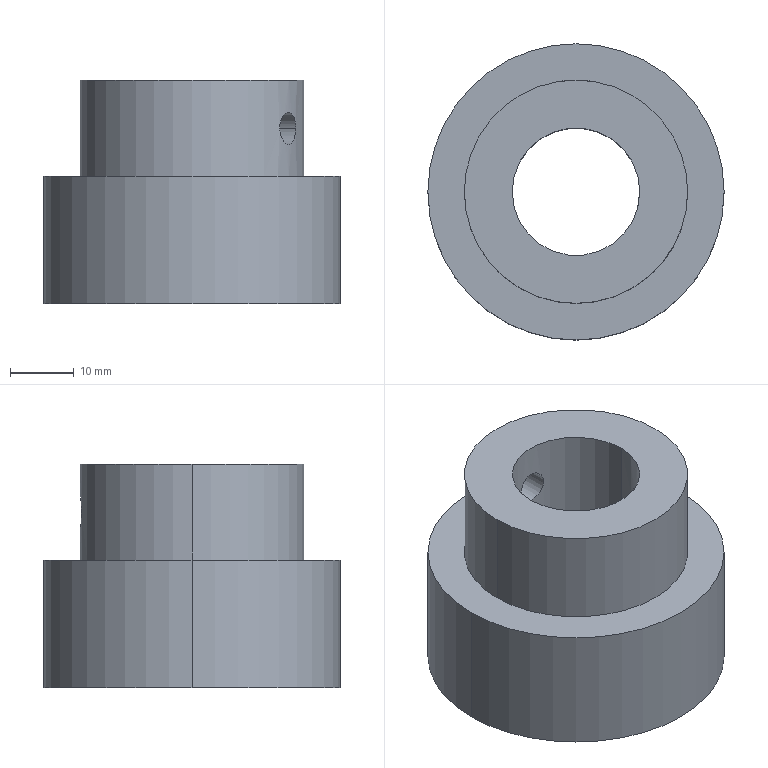Part | SolidWorks | features BaseBody 1 | 1 solid | 13 faces | box 46.43 x 46.43 x 35 mm | volume 37003 mm3 | cylinder 10 | plane 3 | commonest cylinder face diameters 5 x4 20 x2 35 x2 46.43 x2
STEP:
#1=CARTESIAN_POINT('',(7.135,-7.006,27.5));
#2=VERTEX_POINT('',#1);
#3=CARTESIAN_POINT('',(9.635,-2.676,27.5));
#4=VERTEX_POINT('',#3);
#5=CARTESIAN_POINT('',(7.135,-7.006,27.5));
#6=CARTESIAN_POINT('',(7.135,-7.006,27.334));
#7=CARTESIAN_POINT('',(7.147,-6.994,27.171));
#8=CARTESIAN_POINT('',(7.193,-6.947,26.851));
#9=CARTESIAN_POINT('',(7.228,-6.911,26.692));
#10=CARTESIAN_POINT('',(7.316,-6.817,26.389));
#11=CARTESIAN_POINT('',(7.37,-6.76,26.246));
#12=CARTESIAN_POINT('',(7.494,-6.622,25.975));
#13=CARTESIAN_POINT('',(7.565,-6.541,25.847));
#14=CARTESIAN_POINT('',(7.79,-6.274,25.503));
#15=CARTESIAN_POINT('',(7.965,-6.054,25.317));
#16=CARTESIAN_POINT('',(8.228,-5.685,25.129));
#17=CARTESIAN_POINT('',(8.317,-5.554,25.081));
#18=CARTESIAN_POINT('',(8.492,-5.283,25.016));
#19=CARTESIAN_POINT('',(8.577,-5.144,25.));
#20=CARTESIAN_POINT('',(8.741,-4.86,25.));
#21=CARTESIAN_POINT('',(8.821,-4.714,25.016));
#22=CARTESIAN_POINT('',(8.968,-4.428,25.08));
#23=CARTESIAN_POINT('',(9.036,-4.287,25.128));
#24=CARTESIAN_POINT('',(9.225,-3.871,25.316));
#25=CARTESIAN_POINT('',(9.328,-3.612,25.5));
#26=CARTESIAN_POINT('',(9.447,-3.28,25.847));
#27=CARTESIAN_POINT('',(9.481,-3.181,25.973));
#28=CARTESIAN_POINT('',(9.538,-3.005,26.243));
#29=CARTESIAN_POINT('',(9.562,-2.928,26.389));
#30=CARTESIAN_POINT('',(9.599,-2.804,26.691));
#31=CARTESIAN_POINT('',(9.612,-2.757,26.846));
#32=CARTESIAN_POINT('',(9.631,-2.693,27.168));
#33=CARTESIAN_POINT('',(9.635,-2.676,27.334));
#34=CARTESIAN_POINT('',(9.635,-2.676,27.5));
#35=B_SPLINE_CURVE_WITH_KNOTS('',3,(#5,#6,#7,#8,#9,#10,#11,#12,#13,#14,#15,#16,#17,#18,#19,#20,#21,#22,#23,#24,#25,#26,#27,#28,#29,#30,#31,#32,#33,#34),.UNSPECIFIED.,.F.,.F.,(4,2,2,2,2,2,2,2,2,2,2,2,2,2,4),(0.,0.0004903,0.0009806,0.001471,0.001961,0.002942,0.003432,0.003922,0.004413,0.004903,0.005884,0.006374,0.006864,0.007355,0.007845),.UNSPECIFIED.);
#36=EDGE_CURVE('',#2,#4,#35,.T.);
#37=ORIENTED_EDGE('',*,*,#36,.F.);
#38=CARTESIAN_POINT('',(13.75,-10.825,27.5));
#39=VERTEX_POINT('',#38);
#40=CARTESIAN_POINT('',(13.905,-10.915,27.5));
#41=DIRECTION('',(0.866,-0.5,0.));
#42=VECTOR('',#41,1000.);
#43=LINE('',#40,#42);
#44=EDGE_CURVE('',#2,#39,#43,.T.);
#45=ORIENTED_EDGE('',*,*,#44,.T.);
#46=CARTESIAN_POINT('',(16.25,-6.495,27.5));
#47=VERTEX_POINT('',#46);
#48=CARTESIAN_POINT('',(16.25,-6.495,27.5));
#49=CARTESIAN_POINT('',(16.25,-6.495,27.335));
#50=CARTESIAN_POINT('',(16.244,-6.51,27.172));
#51=CARTESIAN_POINT('',(16.22,-6.57,26.852));
#52=CARTESIAN_POINT('',(16.202,-6.615,26.693));
#53=CARTESIAN_POINT('',(16.153,-6.732,26.391));
#54=CARTESIAN_POINT('',(16.124,-6.804,26.247));
#55=CARTESIAN_POINT('',(16.052,-6.972,25.976));
#56=CARTESIAN_POINT('',(16.009,-7.069,25.847));
#57=CARTESIAN_POINT('',(15.914,-7.28,25.617));
#58=CARTESIAN_POINT('',(15.862,-7.395,25.514));
#59=CARTESIAN_POINT('',(15.744,-7.642,25.331));
#60=CARTESIAN_POINT('',(15.68,-7.773,25.253));
#61=CARTESIAN_POINT('',(15.544,-8.041,25.129));
#62=CARTESIAN_POINT('',(15.471,-8.181,25.08));
#63=CARTESIAN_POINT('',(15.317,-8.465,25.016));
#64=CARTESIAN_POINT('',(15.238,-8.607,25.));
#65=CARTESIAN_POINT('',(15.075,-8.89,25.));
#66=CARTESIAN_POINT('',(14.99,-9.032,25.016));
#67=CARTESIAN_POINT('',(14.822,-9.306,25.08));
#68=CARTESIAN_POINT('',(14.738,-9.437,25.127));
#69=CARTESIAN_POINT('',(14.572,-9.691,25.252));
#70=CARTESIAN_POINT('',(14.491,-9.813,25.331));
#71=CARTESIAN_POINT('',(14.337,-10.037,25.511));
#72=CARTESIAN_POINT('',(14.263,-10.14,25.615));
#73=CARTESIAN_POINT('',(14.126,-10.33,25.848));
#74=CARTESIAN_POINT('',(14.064,-10.414,25.974));
#75=CARTESIAN_POINT('',(13.955,-10.56,26.244));
#76=CARTESIAN_POINT('',(13.907,-10.623,26.39));
#77=CARTESIAN_POINT('',(13.83,-10.723,26.693));
#78=CARTESIAN_POINT('',(13.8,-10.761,26.848));
#79=CARTESIAN_POINT('',(13.76,-10.812,27.169));
#80=CARTESIAN_POINT('',(13.75,-10.825,27.335));
#81=CARTESIAN_POINT('',(13.75,-10.825,27.5));
#82=B_SPLINE_CURVE_WITH_KNOTS('',3,(#48,#49,#50,#51,#52,#53,#54,#55,#56,#57,#58,#59,#60,#61,#62,#63,#64,#65,#66,#67,#68,#69,#70,#71,#72,#73,#74,#75,#76,#77,#78,#79,#80,#81),.UNSPECIFIED.,.F.,.F.,(4,2,2,2,2,2,2,2,2,2,2,2,2,2,2,2,4),(0.,0.000489,0.000978,0.001467,0.001956,0.002445,0.002934,0.003423,0.003912,0.004401,0.00489,0.005379,0.005868,0.006357,0.006846,0.007335,0.007824),.UNSPECIFIED.);
#83=EDGE_CURVE('',#47,#39,#82,.T.);
#84=ORIENTED_EDGE('',*,*,#83,.F.);
#85=CARTESIAN_POINT('',(16.405,-6.585,27.5));
#86=DIRECTION('',(0.866,-0.5,0.));
#87=VECTOR('',#86,1000.);
#88=LINE('',#85,#87);
#89=EDGE_CURVE('',#4,#47,#88,.T.);
#90=ORIENTED_EDGE('',*,*,#89,.F.);
#91=EDGE_LOOP('',(#37,#45,#84,#90));
#92=FACE_OUTER_BOUND('',#91,.T.);
#93=CARTESIAN_POINT('',(15.155,-8.75,27.5));
#94=DIRECTION('',(0.866,-0.5,0.));
#95=DIRECTION('',(0.5,0.866,0.));
#96=AXIS2_PLACEMENT_3D('',#93,#94,#95);
#97=CYLINDRICAL_SURFACE('',#96,2.5);
#98=ADVANCED_FACE('',(#92),#97,.F.);
#99=CARTESIAN_POINT('',(0.,10.,25.));
#100=VERTEX_POINT('',#99);
#101=CARTESIAN_POINT('',(0.,10.,30.));
#102=VERTEX_POINT('',#101);
#103=CARTESIAN_POINT('',(0.,10.,25.));
#104=CARTESIAN_POINT('',(-0.1658,10.,25.));
#105=CARTESIAN_POINT('',(-0.3288,9.996,25.016));
#106=CARTESIAN_POINT('',(-0.6491,9.98,25.08));
#107=CARTESIAN_POINT('',(-0.8083,9.968,25.129));
#108=CARTESIAN_POINT('',(-1.111,9.939,25.254));
#109=CARTESIAN_POINT('',(-1.254,9.922,25.331));
#110=CARTESIAN_POINT('',(-1.525,9.884,25.512));
#111=CARTESIAN_POINT('',(-1.653,9.863,25.618));
#112=CARTESIAN_POINT('',(-1.997,9.801,25.962));
#113=CARTESIAN_POINT('',(-2.183,9.76,26.24));
#114=CARTESIAN_POINT('',(-2.371,9.715,26.69));
#115=CARTESIAN_POINT('',(-2.419,9.703,26.848));
#116=CARTESIAN_POINT('',(-2.484,9.687,27.171));
#117=CARTESIAN_POINT('',(-2.5,9.682,27.334));
#118=CARTESIAN_POINT('',(-2.5,9.682,27.661));
#119=CARTESIAN_POINT('',(-2.484,9.687,27.828));
#120=CARTESIAN_POINT('',(-2.42,9.703,28.149));
#121=CARTESIAN_POINT('',(-2.372,9.715,28.305));
#122=CARTESIAN_POINT('',(-2.184,9.759,28.76));
#123=CARTESIAN_POINT('',(-2.,9.801,29.035));
#124=CARTESIAN_POINT('',(-1.653,9.863,29.383));
#125=CARTESIAN_POINT('',(-1.528,9.884,29.486));
#126=CARTESIAN_POINT('',(-1.257,9.922,29.667));
#127=CARTESIAN_POINT('',(-1.111,9.939,29.745));
#128=CARTESIAN_POINT('',(-0.8095,9.968,29.871));
#129=CARTESIAN_POINT('',(-0.6537,9.98,29.919));
#130=CARTESIAN_POINT('',(-0.3318,9.996,29.983));
#131=CARTESIAN_POINT('',(-0.1658,10.,30.));
#132=CARTESIAN_POINT('',(0.,10.,30.));
#133=B_SPLINE_CURVE_WITH_KNOTS('',3,(#103,#104,#105,#106,#107,#108,#109,#110,#111,#112,#113,#114,#115,#116,#117,#118,#119,#120,#121,#122,#123,#124,#125,#126,#127,#128,#129,#130,#131,#132),.UNSPECIFIED.,.F.,.F.,(4,2,2,2,2,2,2,2,2,2,2,2,2,2,4),(0.,0.0004903,0.0009806,0.001471,0.001961,0.002942,0.003432,0.003922,0.004413,0.004903,0.005884,0.006374,0.006864,0.007355,0.007845),.UNSPECIFIED.);
#134=EDGE_CURVE('',#100,#102,#133,.T.);
#135=ORIENTED_EDGE('',*,*,#134,.F.);
#136=CARTESIAN_POINT('',(0.,17.5,25.));
#137=VERTEX_POINT('',#136);
#138=CARTESIAN_POINT('',(0.,17.5,25.));
#139=DIRECTION('',(0.,1.,0.));
#140=VECTOR('',#139,1000.);
#141=LINE('',#138,#140);
#142=EDGE_CURVE('',#100,#137,#141,.T.);
#143=ORIENTED_EDGE('',*,*,#142,.T.);
#144=CARTESIAN_POINT('',(0.,17.5,30.));
#145=VERTEX_POINT('',#144);
#146=CARTESIAN_POINT('',(0.,17.5,30.));
#147=CARTESIAN_POINT('',(-0.1654,17.5,30.));
#148=CARTESIAN_POINT('',(-0.3279,17.498,29.984));
#149=CARTESIAN_POINT('',(-0.6477,17.489,29.92));
#150=CARTESIAN_POINT('',(-0.8066,17.482,29.872));
#151=CARTESIAN_POINT('',(-1.109,17.465,29.746));
#152=CARTESIAN_POINT('',(-1.253,17.456,29.67));
#153=CARTESIAN_POINT('',(-1.524,17.434,29.488));
#154=CARTESIAN_POINT('',(-1.653,17.422,29.383));
#155=CARTESIAN_POINT('',(-1.883,17.399,29.153));
#156=CARTESIAN_POINT('',(-1.986,17.387,29.027));
#157=CARTESIAN_POINT('',(-2.169,17.365,28.754));
#158=CARTESIAN_POINT('',(-2.247,17.355,28.609));
#159=CARTESIAN_POINT('',(-2.371,17.339,28.308));
#160=CARTESIAN_POINT('',(-2.42,17.332,28.15));
#161=CARTESIAN_POINT('',(-2.484,17.323,27.827));
#162=CARTESIAN_POINT('',(-2.5,17.321,27.665));
#163=CARTESIAN_POINT('',(-2.5,17.32,27.339));
#164=CARTESIAN_POINT('',(-2.484,17.323,27.173));
#165=CARTESIAN_POINT('',(-2.42,17.332,26.852));
#166=CARTESIAN_POINT('',(-2.373,17.338,26.696));
#167=CARTESIAN_POINT('',(-2.248,17.355,26.393));
#168=CARTESIAN_POINT('',(-2.169,17.365,26.247));
#169=CARTESIAN_POINT('',(-1.989,17.387,25.976));
#170=CARTESIAN_POINT('',(-1.885,17.399,25.85));
#171=CARTESIAN_POINT('',(-1.652,17.422,25.617));
#172=CARTESIAN_POINT('',(-1.526,17.434,25.513));
#173=CARTESIAN_POINT('',(-1.256,17.455,25.332));
#174=CARTESIAN_POINT('',(-1.11,17.465,25.254));
#175=CARTESIAN_POINT('',(-0.8074,17.482,25.128));
#176=CARTESIAN_POINT('',(-0.6516,17.489,25.081));
#177=CARTESIAN_POINT('',(-0.3309,17.498,25.017));
#178=CARTESIAN_POINT('',(-0.1654,17.5,25.));
#179=CARTESIAN_POINT('',(0.,17.5,25.));
#180=B_SPLINE_CURVE_WITH_KNOTS('',3,(#146,#147,#148,#149,#150,#151,#152,#153,#154,#155,#156,#157,#158,#159,#160,#161,#162,#163,#164,#165,#166,#167,#168,#169,#170,#171,#172,#173,#174,#175,#176,#177,#178,#179),.UNSPECIFIED.,.F.,.F.,(4,2,2,2,2,2,2,2,2,2,2,2,2,2,2,2,4),(0.,0.000489,0.000978,0.001467,0.001956,0.002445,0.002934,0.003423,0.003912,0.004401,0.00489,0.005379,0.005868,0.006357,0.006846,0.007335,0.007824),.UNSPECIFIED.);
#181=EDGE_CURVE('',#145,#137,#180,.T.);
#182=ORIENTED_EDGE('',*,*,#181,.F.);
#183=CARTESIAN_POINT('',(0.,17.5,30.));
#184=DIRECTION('',(0.,1.,0.));
#185=VECTOR('',#184,1000.);
#186=LINE('',#183,#185);
#187=EDGE_CURVE('',#102,#145,#186,.T.);
#188=ORIENTED_EDGE('',*,*,#187,.F.);
#189=EDGE_LOOP('',(#135,#143,#182,#188));
#190=FACE_OUTER_BOUND('',#189,.T.);
#191=CARTESIAN_POINT('',(0.,17.5,27.5));
#192=DIRECTION('',(0.,1.,0.));
#193=DIRECTION('',(0.,0.,1.));
#194=AXIS2_PLACEMENT_3D('',#191,#192,#193);
#195=CYLINDRICAL_SURFACE('',#194,2.5);
#196=ADVANCED_FACE('',(#190),#195,.F.);
#197=CARTESIAN_POINT('',(9.635,-2.676,27.5));
#198=CARTESIAN_POINT('',(9.635,-2.676,27.666));
#199=CARTESIAN_POINT('',(9.631,-2.692,27.829));
#200=CARTESIAN_POINT('',(9.613,-2.756,28.149));
#201=CARTESIAN_POINT('',(9.599,-2.804,28.308));
#202=CARTESIAN_POINT('',(9.562,-2.928,28.611));
#203=CARTESIAN_POINT('',(9.539,-3.003,28.754));
#204=CARTESIAN_POINT('',(9.482,-3.179,29.025));
#205=CARTESIAN_POINT('',(9.447,-3.281,29.153));
#206=CARTESIAN_POINT('',(9.329,-3.61,29.497));
#207=CARTESIAN_POINT('',(9.225,-3.871,29.683));
#208=CARTESIAN_POINT('',(9.038,-4.283,29.871));
#209=CARTESIAN_POINT('',(8.969,-4.426,29.919));
#210=CARTESIAN_POINT('',(8.821,-4.713,29.984));
#211=CARTESIAN_POINT('',(8.743,-4.856,30.));
#212=CARTESIAN_POINT('',(8.58,-5.14,30.));
#213=CARTESIAN_POINT('',(8.493,-5.282,29.984));
#214=CARTESIAN_POINT('',(8.319,-5.552,29.92));
#215=CARTESIAN_POINT('',(8.231,-5.682,29.872));
#216=CARTESIAN_POINT('',(7.965,-6.054,29.684));
#217=CARTESIAN_POINT('',(7.792,-6.272,29.5));
#218=CARTESIAN_POINT('',(7.565,-6.542,29.153));
#219=CARTESIAN_POINT('',(7.495,-6.62,29.027));
#220=CARTESIAN_POINT('',(7.371,-6.758,28.757));
#221=CARTESIAN_POINT('',(7.317,-6.817,28.611));
#222=CARTESIAN_POINT('',(7.228,-6.911,28.309));
#223=CARTESIAN_POINT('',(7.194,-6.946,28.154));
#224=CARTESIAN_POINT('',(7.147,-6.994,27.832));
#225=CARTESIAN_POINT('',(7.135,-7.006,27.666));
#226=CARTESIAN_POINT('',(7.135,-7.006,27.5));
#227=B_SPLINE_CURVE_WITH_KNOTS('',3,(#197,#198,#199,#200,#201,#202,#203,#204,#205,#206,#207,#208,#209,#210,#211,#212,#213,#214,#215,#216,#217,#218,#219,#220,#221,#222,#223,#224,#225,#226),.UNSPECIFIED.,.F.,.F.,(4,2,2,2,2,2,2,2,2,2,2,2,2,2,4),(0.007845,0.008335,0.008825,0.009316,0.009806,0.01079,0.01128,0.01177,0.01226,0.01275,0.01373,0.01422,0.01471,0.0152,0.01569),.UNSPECIFIED.);
#228=EDGE_CURVE('',#4,#2,#227,.T.);
#229=ORIENTED_EDGE('',*,*,#228,.T.);
#230=ORIENTED_EDGE('',*,*,#36,.T.);
#231=EDGE_LOOP('',(#229,#230));
#232=FACE_BOUND('',#231,.T.);
#233=CARTESIAN_POINT('',(-10.,0.,0.));
#234=VERTEX_POINT('',#233);
#235=CARTESIAN_POINT('',(10.,0.,0.));
#236=VERTEX_POINT('',#235);
#237=CARTESIAN_POINT('',(0.,0.,0.));
#238=DIRECTION('',(0.,0.,1.));
#239=DIRECTION('',(1.,0.,0.));
#240=AXIS2_PLACEMENT_3D('',#237,#238,#239);
#241=CIRCLE('',#240,10.);
#242=EDGE_CURVE('',#234,#236,#241,.T.);
#243=ORIENTED_EDGE('',*,*,#242,.F.);
#244=CARTESIAN_POINT('',(-10.,0.,35.));
#245=VERTEX_POINT('',#244);
#246=CARTESIAN_POINT('',(-10.,0.,0.));
#247=DIRECTION('',(0.,0.,1.));
#248=VECTOR('',#247,1000.);
#249=LINE('',#246,#248);
#250=EDGE_CURVE('',#234,#245,#249,.T.);
#251=ORIENTED_EDGE('',*,*,#250,.T.);
#252=CARTESIAN_POINT('',(10.,0.,35.));
#253=VERTEX_POINT('',#252);
#254=CARTESIAN_POINT('',(0.,0.,35.));
#255=DIRECTION('',(0.,0.,1.));
#256=DIRECTION('',(1.,0.,0.));
#257=AXIS2_PLACEMENT_3D('',#254,#255,#256);
#258=CIRCLE('',#257,10.);
#259=EDGE_CURVE('',#245,#253,#258,.T.);
#260=ORIENTED_EDGE('',*,*,#259,.T.);
#261=CARTESIAN_POINT('',(10.,0.,0.));
#262=DIRECTION('',(0.,0.,1.));
#263=VECTOR('',#262,1000.);
#264=LINE('',#261,#263);
#265=EDGE_CURVE('',#236,#253,#264,.T.);
#266=ORIENTED_EDGE('',*,*,#265,.F.);
#267=EDGE_LOOP('',(#243,#251,#260,#266));
#268=FACE_OUTER_BOUND('',#267,.T.);
#269=CARTESIAN_POINT('',(0.,0.,0.));
#270=DIRECTION('',(0.,0.,1.));
#271=DIRECTION('',(1.,0.,0.));
#272=AXIS2_PLACEMENT_3D('',#269,#270,#271);
#273=CYLINDRICAL_SURFACE('',#272,10.);
#274=ADVANCED_FACE('',(#232,#268),#273,.F.);
#275=ORIENTED_EDGE('',*,*,#181,.T.);
#276=CARTESIAN_POINT('',(0.,17.5,25.));
#277=CARTESIAN_POINT('',(0.1654,17.5,25.));
#278=CARTESIAN_POINT('',(0.3279,17.498,25.016));
#279=CARTESIAN_POINT('',(0.6477,17.489,25.08));
#280=CARTESIAN_POINT('',(0.8066,17.482,25.128));
#281=CARTESIAN_POINT('',(1.109,17.465,25.254));
#282=CARTESIAN_POINT('',(1.253,17.456,25.33));
#283=CARTESIAN_POINT('',(1.524,17.434,25.512));
#284=CARTESIAN_POINT('',(1.653,17.422,25.617));
#285=CARTESIAN_POINT('',(1.883,17.399,25.847));
#286=CARTESIAN_POINT('',(1.986,17.387,25.973));
#287=CARTESIAN_POINT('',(2.169,17.365,26.246));
#288=CARTESIAN_POINT('',(2.247,17.355,26.391));
#289=CARTESIAN_POINT('',(2.371,17.339,26.692));
#290=CARTESIAN_POINT('',(2.42,17.332,26.85));
#291=CARTESIAN_POINT('',(2.484,17.323,27.173));
#292=CARTESIAN_POINT('',(2.5,17.321,27.335));
#293=CARTESIAN_POINT('',(2.5,17.32,27.661));
#294=CARTESIAN_POINT('',(2.484,17.323,27.827));
#295=CARTESIAN_POINT('',(2.42,17.332,28.148));
#296=CARTESIAN_POINT('',(2.373,17.338,28.304));
#297=CARTESIAN_POINT('',(2.248,17.355,28.607));
#298=CARTESIAN_POINT('',(2.169,17.365,28.753));
#299=CARTESIAN_POINT('',(1.989,17.387,29.024));
#300=CARTESIAN_POINT('',(1.885,17.399,29.15));
#301=CARTESIAN_POINT('',(1.652,17.422,29.383));
#302=CARTESIAN_POINT('',(1.526,17.434,29.487));
#303=CARTESIAN_POINT('',(1.256,17.455,29.668));
#304=CARTESIAN_POINT('',(1.11,17.465,29.746));
#305=CARTESIAN_POINT('',(0.8074,17.482,29.872));
#306=CARTESIAN_POINT('',(0.6516,17.489,29.919));
#307=CARTESIAN_POINT('',(0.3309,17.498,29.983));
#308=CARTESIAN_POINT('',(0.1654,17.5,30.));
#309=CARTESIAN_POINT('',(0.,17.5,30.));
#310=B_SPLINE_CURVE_WITH_KNOTS('',3,(#276,#277,#278,#279,#280,#281,#282,#283,#284,#285,#286,#287,#288,#289,#290,#291,#292,#293,#294,#295,#296,#297,#298,#299,#300,#301,#302,#303,#304,#305,#306,#307,#308,#309),.UNSPECIFIED.,.F.,.F.,(4,2,2,2,2,2,2,2,2,2,2,2,2,2,2,2,4),(0.007824,0.008313,0.008802,0.009291,0.00978,0.01027,0.01076,0.01125,0.01174,0.01223,0.01271,0.0132,0.01369,0.01418,0.01467,0.01516,0.01565),.UNSPECIFIED.);
#311=EDGE_CURVE('',#137,#145,#310,.T.);
#312=ORIENTED_EDGE('',*,*,#311,.T.);
#313=EDGE_LOOP('',(#275,#312));
#314=FACE_BOUND('',#313,.T.);
#315=CARTESIAN_POINT('',(17.5,0.,35.));
#316=VERTEX_POINT('',#315);
#317=CARTESIAN_POINT('',(-17.5,0.,35.));
#318=VERTEX_POINT('',#317);
#319=CARTESIAN_POINT('',(0.,0.,35.));
#320=DIRECTION('',(0.,0.,1.));
#321=DIRECTION('',(1.,0.,0.));
#322=AXIS2_PLACEMENT_3D('',#319,#320,#321);
#323=CIRCLE('',#322,17.5);
#324=EDGE_CURVE('',#316,#318,#323,.T.);
#325=ORIENTED_EDGE('',*,*,#324,.F.);
#326=CARTESIAN_POINT('',(17.5,0.,20.));
#327=VERTEX_POINT('',#326);
#328=CARTESIAN_POINT('',(17.5,0.,35.));
#329=DIRECTION('',(0.,0.,-1.));
#330=VECTOR('',#329,1000.);
#331=LINE('',#328,#330);
#332=EDGE_CURVE('',#316,#327,#331,.T.);
#333=ORIENTED_EDGE('',*,*,#332,.T.);
#334=CARTESIAN_POINT('',(-17.5,0.,20.));
#335=VERTEX_POINT('',#334);
#336=CARTESIAN_POINT('',(0.,0.,20.));
#337=DIRECTION('',(0.,0.,1.));
#338=DIRECTION('',(1.,0.,0.));
#339=AXIS2_PLACEMENT_3D('',#336,#337,#338);
#340=CIRCLE('',#339,17.5);
#341=EDGE_CURVE('',#327,#335,#340,.T.);
#342=ORIENTED_EDGE('',*,*,#341,.T.);
#343=CARTESIAN_POINT('',(-17.5,0.,35.));
#344=DIRECTION('',(0.,0.,-1.));
#345=VECTOR('',#344,1000.);
#346=LINE('',#343,#345);
#347=EDGE_CURVE('',#318,#335,#346,.T.);
#348=ORIENTED_EDGE('',*,*,#347,.F.);
#349=EDGE_LOOP('',(#325,#333,#342,#348));
#350=FACE_OUTER_BOUND('',#349,.T.);
#351=CARTESIAN_POINT('',(0.,0.,35.));
#352=DIRECTION('',(0.,0.,-1.));
#353=DIRECTION('',(-1.,0.,0.));
#354=AXIS2_PLACEMENT_3D('',#351,#352,#353);
#355=CYLINDRICAL_SURFACE('',#354,17.5);
#356=ADVANCED_FACE('',(#314,#350),#355,.T.);
#357=CARTESIAN_POINT('',(23.215,0.,20.));
#358=VERTEX_POINT('',#357);
#359=CARTESIAN_POINT('',(-23.215,0.,20.));
#360=VERTEX_POINT('',#359);
#361=CARTESIAN_POINT('',(0.,0.,20.));
#362=DIRECTION('',(0.,0.,1.));
#363=DIRECTION('',(1.,0.,0.));
#364=AXIS2_PLACEMENT_3D('',#361,#362,#363);
#365=CIRCLE('',#364,23.215);
#366=EDGE_CURVE('',#358,#360,#365,.T.);
#367=ORIENTED_EDGE('',*,*,#366,.F.);
#368=CARTESIAN_POINT('',(23.215,0.,0.));
#369=VERTEX_POINT('',#368);
#370=CARTESIAN_POINT('',(23.215,0.,20.));
#371=DIRECTION('',(0.,0.,-1.));
#372=VECTOR('',#371,1000.);
#373=LINE('',#370,#372);
#374=EDGE_CURVE('',#358,#369,#373,.T.);
#375=ORIENTED_EDGE('',*,*,#374,.T.);
#376=CARTESIAN_POINT('',(-23.215,0.,0.));
#377=VERTEX_POINT('',#376);
#378=CARTESIAN_POINT('',(0.,0.,0.));
#379=DIRECTION('',(0.,0.,1.));
#380=DIRECTION('',(1.,0.,0.));
#381=AXIS2_PLACEMENT_3D('',#378,#379,#380);
#382=CIRCLE('',#381,23.215);
#383=EDGE_CURVE('',#369,#377,#382,.T.);
#384=ORIENTED_EDGE('',*,*,#383,.T.);
#385=CARTESIAN_POINT('',(-23.215,0.,20.));
#386=DIRECTION('',(0.,0.,-1.));
#387=VECTOR('',#386,1000.);
#388=LINE('',#385,#387);
#389=EDGE_CURVE('',#360,#377,#388,.T.);
#390=ORIENTED_EDGE('',*,*,#389,.F.);
#391=EDGE_LOOP('',(#367,#375,#384,#390));
#392=FACE_OUTER_BOUND('',#391,.T.);
#393=CARTESIAN_POINT('',(0.,0.,20.));
#394=DIRECTION('',(0.,0.,-1.));
#395=DIRECTION('',(-1.,0.,0.));
#396=AXIS2_PLACEMENT_3D('',#393,#394,#395);
#397=CYLINDRICAL_SURFACE('',#396,23.215);
#398=ADVANCED_FACE('',(#392),#397,.T.);
#399=CARTESIAN_POINT('',(0.,0.,35.));
#400=DIRECTION('',(0.,0.,1.));
#401=DIRECTION('',(1.,0.,0.));
#402=AXIS2_PLACEMENT_3D('',#399,#400,#401);
#403=CIRCLE('',#402,10.);
#404=EDGE_CURVE('',#253,#245,#403,.T.);
#405=ORIENTED_EDGE('',*,*,#404,.F.);
#406=ORIENTED_EDGE('',*,*,#259,.F.);
#407=EDGE_LOOP('',(#405,#406));
#408=FACE_BOUND('',#407,.T.);
#409=CARTESIAN_POINT('',(0.,0.,35.));
#410=DIRECTION('',(0.,0.,1.));
#411=DIRECTION('',(1.,0.,0.));
#412=AXIS2_PLACEMENT_3D('',#409,#410,#411);
#413=CIRCLE('',#412,17.5);
#414=EDGE_CURVE('',#318,#316,#413,.T.);
#415=ORIENTED_EDGE('',*,*,#414,.T.);
#416=ORIENTED_EDGE('',*,*,#324,.T.);
#417=EDGE_LOOP('',(#415,#416));
#418=FACE_OUTER_BOUND('',#417,.T.);
#419=CARTESIAN_POINT('',(0.,0.,35.));
#420=DIRECTION('',(0.,0.,1.));
#421=DIRECTION('',(0.,-1.,0.));
#422=AXIS2_PLACEMENT_3D('',#419,#420,#421);
#423=PLANE('',#422);
#424=ADVANCED_FACE('',(#408,#418),#423,.T.);
#425=CARTESIAN_POINT('',(0.,0.,0.));
#426=DIRECTION('',(0.,0.,1.));
#427=DIRECTION('',(1.,0.,0.));
#428=AXIS2_PLACEMENT_3D('',#425,#426,#427);
#429=CIRCLE('',#428,10.);
#430=EDGE_CURVE('',#236,#234,#429,.T.);
#431=ORIENTED_EDGE('',*,*,#430,.T.);
#432=ORIENTED_EDGE('',*,*,#242,.T.);
#433=EDGE_LOOP('',(#431,#432));
#434=FACE_BOUND('',#433,.T.);
#435=CARTESIAN_POINT('',(0.,0.,0.));
#436=DIRECTION('',(0.,0.,1.));
#437=DIRECTION('',(1.,0.,0.));
#438=AXIS2_PLACEMENT_3D('',#435,#436,#437);
#439=CIRCLE('',#438,23.215);
#440=EDGE_CURVE('',#377,#369,#439,.T.);
#441=ORIENTED_EDGE('',*,*,#440,.F.);
#442=ORIENTED_EDGE('',*,*,#383,.F.);
#443=EDGE_LOOP('',(#441,#442));
#444=FACE_OUTER_BOUND('',#443,.T.);
#445=CARTESIAN_POINT('',(0.,0.,0.));
#446=DIRECTION('',(0.,0.,1.));
#447=DIRECTION('',(0.,-1.,0.));
#448=AXIS2_PLACEMENT_3D('',#445,#446,#447);
#449=PLANE('',#448);
#450=ADVANCED_FACE('',(#434,#444),#449,.F.);
#451=CARTESIAN_POINT('',(0.,0.,20.));
#452=DIRECTION('',(0.,0.,1.));
#453=DIRECTION('',(1.,0.,0.));
#454=AXIS2_PLACEMENT_3D('',#451,#452,#453);
#455=CIRCLE('',#454,17.5);
#456=EDGE_CURVE('',#335,#327,#455,.T.);
#457=ORIENTED_EDGE('',*,*,#456,.F.);
#458=ORIENTED_EDGE('',*,*,#341,.F.);
#459=EDGE_LOOP('',(#457,#458));
#460=FACE_BOUND('',#459,.T.);
#461=CARTESIAN_POINT('',(0.,0.,20.));
#462=DIRECTION('',(0.,0.,1.));
#463=DIRECTION('',(1.,0.,0.));
#464=AXIS2_PLACEMENT_3D('',#461,#462,#463);
#465=CIRCLE('',#464,23.215);
#466=EDGE_CURVE('',#360,#358,#465,.T.);
#467=ORIENTED_EDGE('',*,*,#466,.T.);
#468=ORIENTED_EDGE('',*,*,#366,.T.);
#469=EDGE_LOOP('',(#467,#468));
#470=FACE_OUTER_BOUND('',#469,.T.);
#471=CARTESIAN_POINT('',(0.,0.,20.));
#472=DIRECTION('',(0.,0.,1.));
#473=DIRECTION('',(0.,-1.,0.));
#474=AXIS2_PLACEMENT_3D('',#471,#472,#473);
#475=PLANE('',#474);
#476=ADVANCED_FACE('',(#460,#470),#475,.T.);
#477=ORIENTED_EDGE('',*,*,#374,.F.);
#478=ORIENTED_EDGE('',*,*,#466,.F.);
#479=ORIENTED_EDGE('',*,*,#389,.T.);
#480=ORIENTED_EDGE('',*,*,#440,.T.);
#481=EDGE_LOOP('',(#477,#478,#479,#480));
#482=FACE_OUTER_BOUND('',#481,.T.);
#483=CARTESIAN_POINT('',(0.,0.,20.));
#484=DIRECTION('',(0.,0.,-1.));
#485=DIRECTION('',(-1.,0.,0.));
#486=AXIS2_PLACEMENT_3D('',#483,#484,#485);
#487=CYLINDRICAL_SURFACE('',#486,23.215);
#488=ADVANCED_FACE('',(#482),#487,.T.);
#489=ORIENTED_EDGE('',*,*,#332,.F.);
#490=ORIENTED_EDGE('',*,*,#414,.F.);
#491=ORIENTED_EDGE('',*,*,#347,.T.);
#492=ORIENTED_EDGE('',*,*,#456,.T.);
#493=EDGE_LOOP('',(#489,#490,#491,#492));
#494=FACE_OUTER_BOUND('',#493,.T.);
#495=ORIENTED_EDGE('',*,*,#83,.T.);
#496=CARTESIAN_POINT('',(13.75,-10.825,27.5));
#497=CARTESIAN_POINT('',(13.75,-10.825,27.665));
#498=CARTESIAN_POINT('',(13.76,-10.812,27.828));
#499=CARTESIAN_POINT('',(13.8,-10.762,28.148));
#500=CARTESIAN_POINT('',(13.83,-10.724,28.307));
#501=CARTESIAN_POINT('',(13.907,-10.623,28.609));
#502=CARTESIAN_POINT('',(13.954,-10.562,28.753));
#503=CARTESIAN_POINT('',(14.063,-10.415,29.024));
#504=CARTESIAN_POINT('',(14.126,-10.33,29.153));
#505=CARTESIAN_POINT('',(14.262,-10.142,29.383));
#506=CARTESIAN_POINT('',(14.335,-10.039,29.486));
#507=CARTESIAN_POINT('',(14.49,-9.814,29.669));
#508=CARTESIAN_POINT('',(14.571,-9.693,29.747));
#509=CARTESIAN_POINT('',(14.736,-9.441,29.871));
#510=CARTESIAN_POINT('',(14.821,-9.307,29.92));
#511=CARTESIAN_POINT('',(14.99,-9.032,29.984));
#512=CARTESIAN_POINT('',(15.073,-8.893,30.));
#513=CARTESIAN_POINT('',(15.236,-8.61,30.));
#514=CARTESIAN_POINT('',(15.317,-8.465,29.984));
#515=CARTESIAN_POINT('',(15.47,-8.183,29.92));
#516=CARTESIAN_POINT('',(15.542,-8.045,29.873));
#517=CARTESIAN_POINT('',(15.679,-7.774,29.748));
#518=CARTESIAN_POINT('',(15.743,-7.643,29.669));
#519=CARTESIAN_POINT('',(15.86,-7.398,29.489));
#520=CARTESIAN_POINT('',(15.913,-7.282,29.385));
#521=CARTESIAN_POINT('',(16.009,-7.068,29.152));
#522=CARTESIAN_POINT('',(16.051,-6.973,29.026));
#523=CARTESIAN_POINT('',(16.123,-6.805,28.756));
#524=CARTESIAN_POINT('',(16.153,-6.732,28.61));
#525=CARTESIAN_POINT('',(16.202,-6.615,28.307));
#526=CARTESIAN_POINT('',(16.22,-6.571,28.152));
#527=CARTESIAN_POINT('',(16.244,-6.511,27.831));
#528=CARTESIAN_POINT('',(16.25,-6.495,27.665));
#529=CARTESIAN_POINT('',(16.25,-6.495,27.5));
#530=B_SPLINE_CURVE_WITH_KNOTS('',3,(#496,#497,#498,#499,#500,#501,#502,#503,#504,#505,#506,#507,#508,#509,#510,#511,#512,#513,#514,#515,#516,#517,#518,#519,#520,#521,#522,#523,#524,#525,#526,#527,#528,#529),.UNSPECIFIED.,.F.,.F.,(4,2,2,2,2,2,2,2,2,2,2,2,2,2,2,2,4),(0.007824,0.008313,0.008802,0.009291,0.00978,0.01027,0.01076,0.01125,0.01174,0.01223,0.01271,0.0132,0.01369,0.01418,0.01467,0.01516,0.01565),.UNSPECIFIED.);
#531=EDGE_CURVE('',#39,#47,#530,.T.);
#532=ORIENTED_EDGE('',*,*,#531,.T.);
#533=EDGE_LOOP('',(#495,#532));
#534=FACE_BOUND('',#533,.T.);
#535=CARTESIAN_POINT('',(0.,0.,35.));
#536=DIRECTION('',(0.,0.,-1.));
#537=DIRECTION('',(-1.,0.,0.));
#538=AXIS2_PLACEMENT_3D('',#535,#536,#537);
#539=CYLINDRICAL_SURFACE('',#538,17.5);
#540=ADVANCED_FACE('',(#494,#534),#539,.T.);
#541=ORIENTED_EDGE('',*,*,#250,.F.);
#542=ORIENTED_EDGE('',*,*,#430,.F.);
#543=ORIENTED_EDGE('',*,*,#265,.T.);
#544=ORIENTED_EDGE('',*,*,#404,.T.);
#545=EDGE_LOOP('',(#541,#542,#543,#544));
#546=FACE_OUTER_BOUND('',#545,.T.);
#547=CARTESIAN_POINT('',(0.,10.,30.));
#548=CARTESIAN_POINT('',(0.1658,10.,30.));
#549=CARTESIAN_POINT('',(0.3288,9.996,29.984));
#550=CARTESIAN_POINT('',(0.6491,9.98,29.92));
#551=CARTESIAN_POINT('',(0.8083,9.968,29.871));
#552=CARTESIAN_POINT('',(1.111,9.939,29.746));
#553=CARTESIAN_POINT('',(1.254,9.922,29.669));
#554=CARTESIAN_POINT('',(1.525,9.884,29.488));
#555=CARTESIAN_POINT('',(1.653,9.863,29.382));
#556=CARTESIAN_POINT('',(1.997,9.801,29.038));
#557=CARTESIAN_POINT('',(2.183,9.76,28.76));
#558=CARTESIAN_POINT('',(2.371,9.715,28.31));
#559=CARTESIAN_POINT('',(2.419,9.703,28.152));
#560=CARTESIAN_POINT('',(2.484,9.687,27.829));
#561=CARTESIAN_POINT('',(2.5,9.682,27.666));
#562=CARTESIAN_POINT('',(2.5,9.682,27.339));
#563=CARTESIAN_POINT('',(2.484,9.687,27.172));
#564=CARTESIAN_POINT('',(2.42,9.703,26.851));
#565=CARTESIAN_POINT('',(2.372,9.715,26.695));
#566=CARTESIAN_POINT('',(2.184,9.759,26.24));
#567=CARTESIAN_POINT('',(2.,9.801,25.965));
#568=CARTESIAN_POINT('',(1.653,9.863,25.617));
#569=CARTESIAN_POINT('',(1.528,9.884,25.514));
#570=CARTESIAN_POINT('',(1.257,9.922,25.333));
#571=CARTESIAN_POINT('',(1.111,9.939,25.255));
#572=CARTESIAN_POINT('',(0.8095,9.968,25.129));
#573=CARTESIAN_POINT('',(0.6537,9.98,25.081));
#574=CARTESIAN_POINT('',(0.3318,9.996,25.017));
#575=CARTESIAN_POINT('',(0.1658,10.,25.));
#576=CARTESIAN_POINT('',(0.,10.,25.));
#577=B_SPLINE_CURVE_WITH_KNOTS('',3,(#547,#548,#549,#550,#551,#552,#553,#554,#555,#556,#557,#558,#559,#560,#561,#562,#563,#564,#565,#566,#567,#568,#569,#570,#571,#572,#573,#574,#575,#576),.UNSPECIFIED.,.F.,.F.,(4,2,2,2,2,2,2,2,2,2,2,2,2,2,4),(0.007845,0.008335,0.008826,0.009316,0.009806,0.01079,0.01128,0.01177,0.01226,0.01275,0.01373,0.01422,0.01471,0.0152,0.01569),.UNSPECIFIED.);
#578=EDGE_CURVE('',#102,#100,#577,.T.);
#579=ORIENTED_EDGE('',*,*,#578,.T.);
#580=ORIENTED_EDGE('',*,*,#134,.T.);
#581=EDGE_LOOP('',(#579,#580));
#582=FACE_BOUND('',#581,.T.);
#583=CARTESIAN_POINT('',(0.,0.,0.));
#584=DIRECTION('',(0.,0.,1.));
#585=DIRECTION('',(1.,0.,0.));
#586=AXIS2_PLACEMENT_3D('',#583,#584,#585);
#587=CYLINDRICAL_SURFACE('',#586,10.);
#588=ADVANCED_FACE('',(#546,#582),#587,.F.);
#589=ORIENTED_EDGE('',*,*,#142,.F.);
#590=ORIENTED_EDGE('',*,*,#578,.F.);
#591=ORIENTED_EDGE('',*,*,#187,.T.);
#592=ORIENTED_EDGE('',*,*,#311,.F.);
#593=EDGE_LOOP('',(#589,#590,#591,#592));
#594=FACE_OUTER_BOUND('',#593,.T.);
#595=CARTESIAN_POINT('',(0.,17.5,27.5));
#596=DIRECTION('',(0.,1.,0.));
#597=DIRECTION('',(0.,0.,1.));
#598=AXIS2_PLACEMENT_3D('',#595,#596,#597);
#599=CYLINDRICAL_SURFACE('',#598,2.5);
#600=ADVANCED_FACE('',(#594),#599,.F.);
#601=ORIENTED_EDGE('',*,*,#44,.F.);
#602=ORIENTED_EDGE('',*,*,#228,.F.);
#603=ORIENTED_EDGE('',*,*,#89,.T.);
#604=ORIENTED_EDGE('',*,*,#531,.F.);
#605=EDGE_LOOP('',(#601,#602,#603,#604));
#606=FACE_OUTER_BOUND('',#605,.T.);
#607=CARTESIAN_POINT('',(15.155,-8.75,27.5));
#608=DIRECTION('',(0.866,-0.5,0.));
#609=DIRECTION('',(0.5,0.866,0.));
#610=AXIS2_PLACEMENT_3D('',#607,#608,#609);
#611=CYLINDRICAL_SURFACE('',#610,2.5);
#612=ADVANCED_FACE('',(#606),#611,.F.);
#613=CLOSED_SHELL('',(#98,#196,#274,#356,#398,#424,#450,#476,#488,#540,#588,#600,#612));
#614=MANIFOLD_SOLID_BREP('',#613);
#615=CARTESIAN_POINT('',(0.,0.,0.));
#616=DIRECTION('',(0.,0.,1.));
#617=DIRECTION('',(1.,0.,0.));
#618=AXIS2_PLACEMENT_3D('',#615,#616,#617);
#619=(LENGTH_UNIT()NAMED_UNIT(*)SI_UNIT(.MILLI.,.METRE.));
#620=UNCERTAINTY_MEASURE_WITH_UNIT(LENGTH_MEASURE(0.00001),#619,'','');
#621=(NAMED_UNIT(*)PLANE_ANGLE_UNIT()SI_UNIT($,.RADIAN.));
#622=(NAMED_UNIT(*)SI_UNIT($,.STERADIAN.)SOLID_ANGLE_UNIT());
#623=(GEOMETRIC_REPRESENTATION_CONTEXT(3)GLOBAL_UNCERTAINTY_ASSIGNED_CONTEXT((#620))GLOBAL_UNIT_ASSIGNED_CONTEXT((#619,#621,#622))REPRESENTATION_CONTEXT('',''));
#624=ADVANCED_BREP_SHAPE_REPRESENTATION('',(#614,#618),#623);